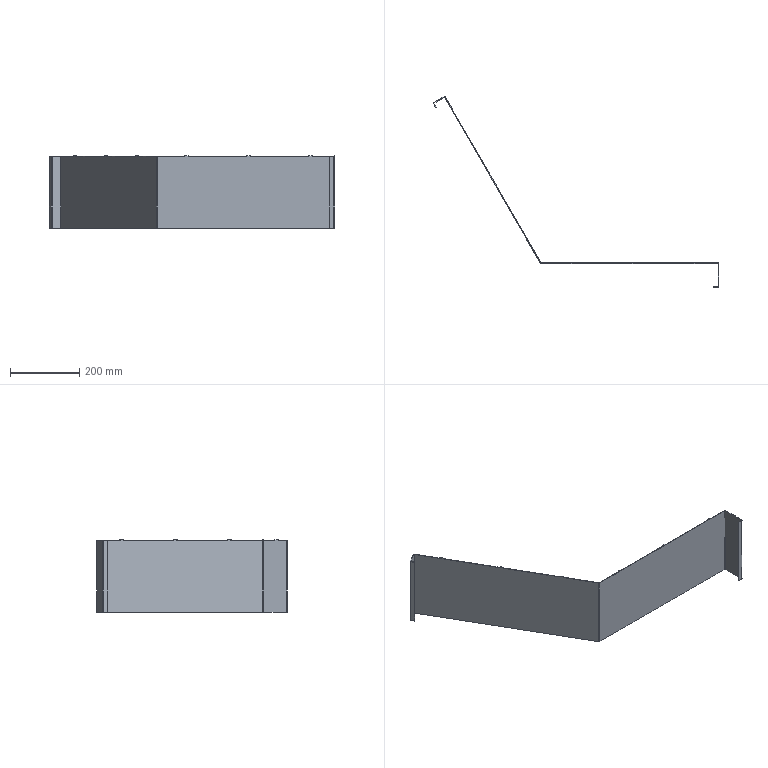Part | STEP file | zh002 | 1 solid | 56 faces | box 827.795 x 553.29 x 210 mm | volume 501438 mm3 | plane 44 | cylinder 12 | commonest cylinder face diameters 1 x6 5 x6